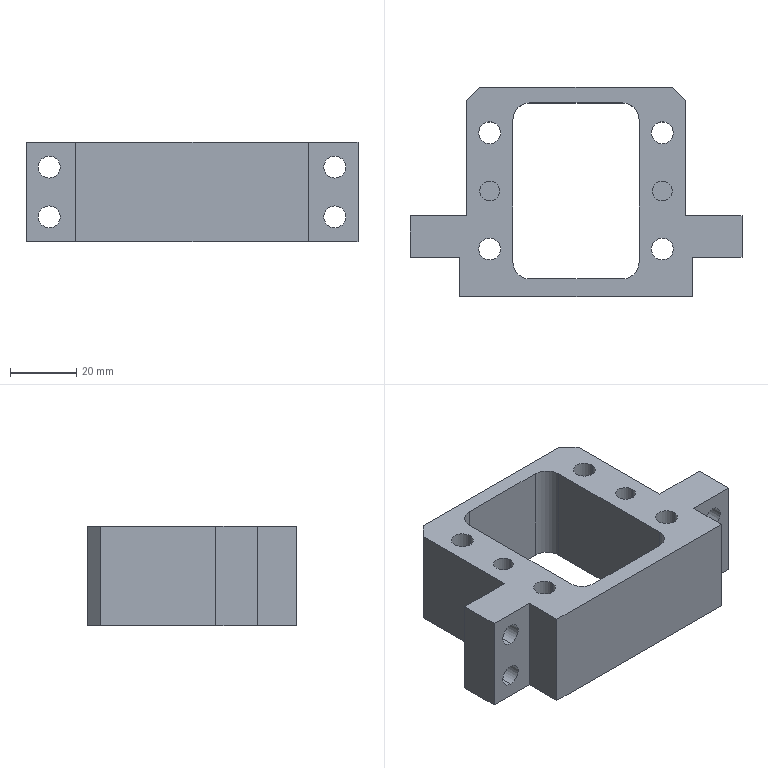Part | SolidWorks | features BaseBody 1 | 1 solid | 78 faces | box 100 x 63 x 30 mm | volume 67109 mm3 | cylinder 44 | plane 30 | cone 4 | commonest cylinder face diameters 6.6 x16 11 x16 2.5 x4 6 x4 10 x4